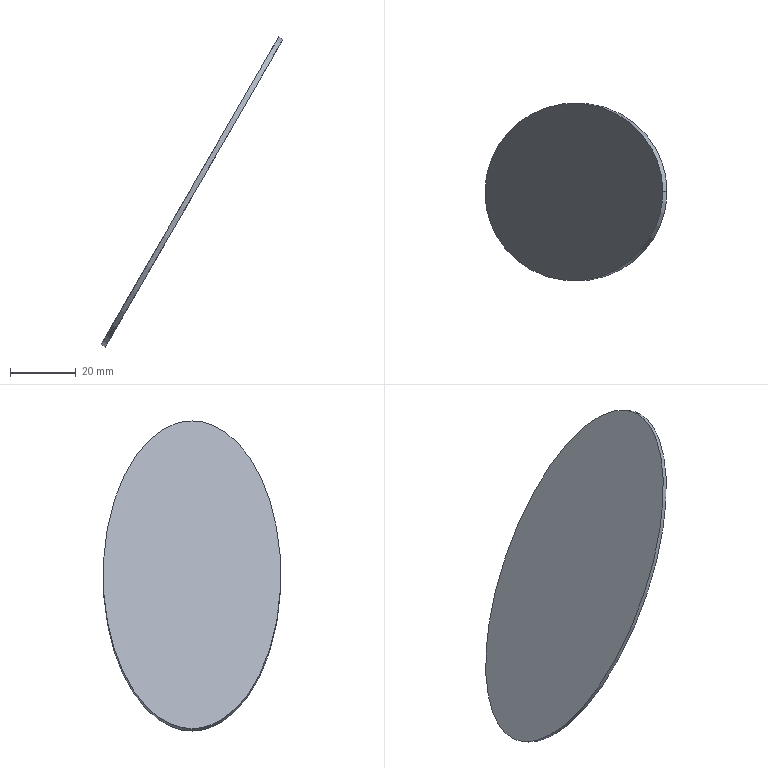Part | SolidWorks | features ICE 4, Extrusion 1 | 1 solid | 4 faces | box 55.199 x 53.9 x 94.108 mm | volume 6846 mm3 | spline 2 | plane 2
STEP:
#1=CARTESIAN_POINT('',(-26.517,0.,0.234));
#2=VERTEX_POINT('',#1);
#3=CARTESIAN_POINT('',(27.383,0.,93.592));
#4=VERTEX_POINT('',#3);
#5=CARTESIAN_POINT('',(-26.517,0.,0.234));
#6=CARTESIAN_POINT('',(-26.517,53.9,0.234));
#7=CARTESIAN_POINT('',(27.383,53.9,93.592));
#8=CARTESIAN_POINT('',(27.383,0.,93.592));
#9=(BOUNDED_CURVE()B_SPLINE_CURVE(3,(#5,#6,#7,#8),.UNSPECIFIED.,.F.,.T.)B_SPLINE_CURVE_WITH_KNOTS((4,4),(0.,3.142),.UNSPECIFIED.)CURVE()GEOMETRIC_REPRESENTATION_ITEM()RATIONAL_B_SPLINE_CURVE((1.,0.3333,0.3333,1.))REPRESENTATION_ITEM(''));
#10=EDGE_CURVE('',#2,#4,#9,.T.);
#11=ORIENTED_EDGE('',*,*,#10,.T.);
#12=CARTESIAN_POINT('',(28.682,0.,92.842));
#13=VERTEX_POINT('',#12);
#14=CARTESIAN_POINT('',(-5.093,0.,112.342));
#15=DIRECTION('',(0.866,0.,-0.5));
#16=VECTOR('',#15,1000.);
#17=LINE('',#14,#16);
#18=EDGE_CURVE('',#4,#13,#17,.T.);
#19=ORIENTED_EDGE('',*,*,#18,.T.);
#20=CARTESIAN_POINT('',(-25.218,0.,-0.516));
#21=VERTEX_POINT('',#20);
#22=CARTESIAN_POINT('',(-25.218,0.,-0.516));
#23=CARTESIAN_POINT('',(-25.218,53.9,-0.516));
#24=CARTESIAN_POINT('',(28.682,53.9,92.842));
#25=CARTESIAN_POINT('',(28.682,0.,92.842));
#26=(BOUNDED_CURVE()B_SPLINE_CURVE(3,(#22,#23,#24,#25),.UNSPECIFIED.,.F.,.T.)B_SPLINE_CURVE_WITH_KNOTS((4,4),(0.,3.142),.UNSPECIFIED.)CURVE()GEOMETRIC_REPRESENTATION_ITEM()RATIONAL_B_SPLINE_CURVE((1.,0.3333,0.3333,1.))REPRESENTATION_ITEM(''));
#27=EDGE_CURVE('',#21,#13,#26,.T.);
#28=ORIENTED_EDGE('',*,*,#27,.F.);
#29=CARTESIAN_POINT('',(-58.993,0.,18.984));
#30=DIRECTION('',(0.866,0.,-0.5));
#31=VECTOR('',#30,1000.);
#32=LINE('',#29,#31);
#33=EDGE_CURVE('',#2,#21,#32,.T.);
#34=ORIENTED_EDGE('',*,*,#33,.F.);
#35=EDGE_LOOP('',(#11,#19,#28,#34));
#36=FACE_OUTER_BOUND('',#35,.T.);
#37=CARTESIAN_POINT('',(-26.517,0.,0.234));
#38=CARTESIAN_POINT('',(-25.218,0.,-0.516));
#39=CARTESIAN_POINT('',(-26.517,53.9,0.234));
#40=CARTESIAN_POINT('',(-25.218,53.9,-0.516));
#41=CARTESIAN_POINT('',(27.383,53.9,93.592));
#42=CARTESIAN_POINT('',(28.682,53.9,92.842));
#43=CARTESIAN_POINT('',(27.383,0.,93.592));
#44=CARTESIAN_POINT('',(28.682,0.,92.842));
#45=(BOUNDED_SURFACE()B_SPLINE_SURFACE(3,1,((#37,#38),(#39,#40),(#41,#42),(#43,#44)),.UNSPECIFIED.,.F.,.F.,.F.)B_SPLINE_SURFACE_WITH_KNOTS((4,4),(2,2),(0.,1.),(0.,1.),.UNSPECIFIED.)GEOMETRIC_REPRESENTATION_ITEM()RATIONAL_B_SPLINE_SURFACE(((1.,1.),(0.3333,0.3333),(0.3333,0.3333),(1.,1.)))REPRESENTATION_ITEM('')SURFACE());
#46=ADVANCED_FACE('',(#36),#45,.T.);
#47=ORIENTED_EDGE('',*,*,#18,.F.);
#48=CARTESIAN_POINT('',(27.383,0.,93.592));
#49=CARTESIAN_POINT('',(27.383,-53.9,93.592));
#50=CARTESIAN_POINT('',(-26.517,-53.9,0.234));
#51=CARTESIAN_POINT('',(-26.517,0.,0.234));
#52=(BOUNDED_CURVE()B_SPLINE_CURVE(3,(#48,#49,#50,#51),.UNSPECIFIED.,.F.,.T.)B_SPLINE_CURVE_WITH_KNOTS((4,4),(3.142,6.283),.UNSPECIFIED.)CURVE()GEOMETRIC_REPRESENTATION_ITEM()RATIONAL_B_SPLINE_CURVE((1.,0.3333,0.3333,1.))REPRESENTATION_ITEM(''));
#53=EDGE_CURVE('',#4,#2,#52,.T.);
#54=ORIENTED_EDGE('',*,*,#53,.T.);
#55=ORIENTED_EDGE('',*,*,#33,.T.);
#56=CARTESIAN_POINT('',(28.682,0.,92.842));
#57=CARTESIAN_POINT('',(28.682,-53.9,92.842));
#58=CARTESIAN_POINT('',(-25.218,-53.9,-0.516));
#59=CARTESIAN_POINT('',(-25.218,0.,-0.516));
#60=(BOUNDED_CURVE()B_SPLINE_CURVE(3,(#56,#57,#58,#59),.UNSPECIFIED.,.F.,.T.)B_SPLINE_CURVE_WITH_KNOTS((4,4),(3.142,6.283),.UNSPECIFIED.)CURVE()GEOMETRIC_REPRESENTATION_ITEM()RATIONAL_B_SPLINE_CURVE((1.,0.3333,0.3333,1.))REPRESENTATION_ITEM(''));
#61=EDGE_CURVE('',#13,#21,#60,.T.);
#62=ORIENTED_EDGE('',*,*,#61,.F.);
#63=EDGE_LOOP('',(#47,#54,#55,#62));
#64=FACE_OUTER_BOUND('',#63,.T.);
#65=CARTESIAN_POINT('',(27.383,0.,93.592));
#66=CARTESIAN_POINT('',(28.682,0.,92.842));
#67=CARTESIAN_POINT('',(27.383,-53.9,93.592));
#68=CARTESIAN_POINT('',(28.682,-53.9,92.842));
#69=CARTESIAN_POINT('',(-26.517,-53.9,0.234));
#70=CARTESIAN_POINT('',(-25.218,-53.9,-0.516));
#71=CARTESIAN_POINT('',(-26.517,0.,0.234));
#72=CARTESIAN_POINT('',(-25.218,0.,-0.516));
#73=(BOUNDED_SURFACE()B_SPLINE_SURFACE(3,1,((#65,#66),(#67,#68),(#69,#70),(#71,#72)),.UNSPECIFIED.,.F.,.F.,.T.)B_SPLINE_SURFACE_WITH_KNOTS((4,4),(2,2),(0.,1.),(0.,1.),.UNSPECIFIED.)GEOMETRIC_REPRESENTATION_ITEM()RATIONAL_B_SPLINE_SURFACE(((1.,1.),(0.3333,0.3333),(0.3333,0.3333),(1.,1.)))REPRESENTATION_ITEM('')SURFACE());
#74=ADVANCED_FACE('',(#64),#73,.T.);
#75=ORIENTED_EDGE('',*,*,#27,.T.);
#76=ORIENTED_EDGE('',*,*,#61,.T.);
#77=EDGE_LOOP('',(#75,#76));
#78=FACE_OUTER_BOUND('',#77,.T.);
#79=CARTESIAN_POINT('',(1.732,0.,46.163));
#80=DIRECTION('',(0.866,0.,-0.5));
#81=DIRECTION('',(-0.5,0.,-0.866));
#82=AXIS2_PLACEMENT_3D('',#79,#80,#81);
#83=PLANE('',#82);
#84=ADVANCED_FACE('',(#78),#83,.T.);
#85=ORIENTED_EDGE('',*,*,#10,.F.);
#86=ORIENTED_EDGE('',*,*,#53,.F.);
#87=EDGE_LOOP('',(#85,#86));
#88=FACE_OUTER_BOUND('',#87,.T.);
#89=CARTESIAN_POINT('',(0.433,0.,46.913));
#90=DIRECTION('',(0.866,0.,-0.5));
#91=DIRECTION('',(-0.5,0.,-0.866));
#92=AXIS2_PLACEMENT_3D('',#89,#90,#91);
#93=PLANE('',#92);
#94=ADVANCED_FACE('',(#88),#93,.F.);
#95=CLOSED_SHELL('',(#46,#74,#84,#94));
#96=MANIFOLD_SOLID_BREP('',#95);
#97=CARTESIAN_POINT('',(0.,0.,0.));
#98=DIRECTION('',(0.,0.,1.));
#99=DIRECTION('',(1.,0.,0.));
#100=AXIS2_PLACEMENT_3D('',#97,#98,#99);
#101=(LENGTH_UNIT()NAMED_UNIT(*)SI_UNIT(.MILLI.,.METRE.));
#102=UNCERTAINTY_MEASURE_WITH_UNIT(LENGTH_MEASURE(0.00001),#101,'','');
#103=(NAMED_UNIT(*)PLANE_ANGLE_UNIT()SI_UNIT($,.RADIAN.));
#104=(NAMED_UNIT(*)SI_UNIT($,.STERADIAN.)SOLID_ANGLE_UNIT());
#105=(GEOMETRIC_REPRESENTATION_CONTEXT(3)GLOBAL_UNCERTAINTY_ASSIGNED_CONTEXT((#102))GLOBAL_UNIT_ASSIGNED_CONTEXT((#101,#103,#104))REPRESENTATION_CONTEXT('',''));
#106=ADVANCED_BREP_SHAPE_REPRESENTATION('',(#96,#100),#105);